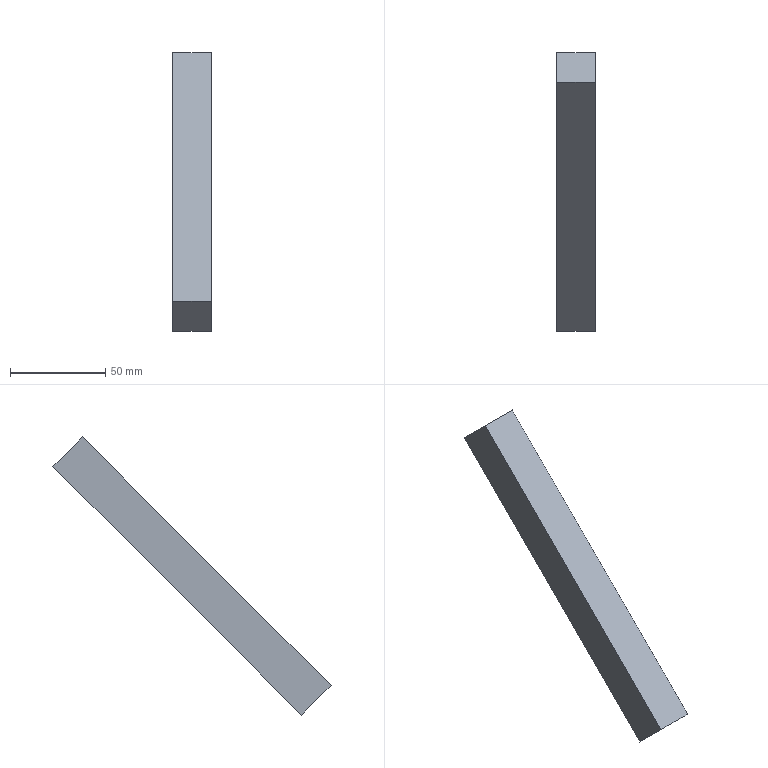Part | NX | features solid 2 | 1 solid | 6 faces | box 20 x 145.664 x 145.664 mm | volume 80960 mm3 | plane 6
STEP:
#1=CARTESIAN_POINT('',(-110.,-290.882,-104.607));
#2=VERTEX_POINT('',#1);
#3=CARTESIAN_POINT('',(-110.,-160.775,25.5));
#4=VERTEX_POINT('',#3);
#5=CARTESIAN_POINT('',(-110.,-282.751,-96.475));
#6=DIRECTION('',(0.,0.7071,0.7071));
#7=VECTOR('',#6,1000.);
#8=LINE('',#5,#7);
#9=EDGE_CURVE('',#2,#4,#8,.T.);
#10=ORIENTED_EDGE('',*,*,#9,.F.);
#11=CARTESIAN_POINT('',(-130.,-290.882,-104.607));
#12=VERTEX_POINT('',#11);
#13=CARTESIAN_POINT('',(-130.,-290.882,-104.607));
#14=DIRECTION('',(1.,0.,0.));
#15=VECTOR('',#14,1000.);
#16=LINE('',#13,#15);
#17=EDGE_CURVE('',#12,#2,#16,.T.);
#18=ORIENTED_EDGE('',*,*,#17,.F.);
#19=CARTESIAN_POINT('',(-130.,-160.775,25.5));
#20=VERTEX_POINT('',#19);
#21=CARTESIAN_POINT('',(-130.,-282.751,-96.475));
#22=DIRECTION('',(0.,0.7071,0.7071));
#23=VECTOR('',#22,1000.);
#24=LINE('',#21,#23);
#25=EDGE_CURVE('',#12,#20,#24,.T.);
#26=ORIENTED_EDGE('',*,*,#25,.T.);
#27=CARTESIAN_POINT('',(-130.,-160.775,25.5));
#28=DIRECTION('',(1.,0.,0.));
#29=VECTOR('',#28,1000.);
#30=LINE('',#27,#29);
#31=EDGE_CURVE('',#20,#4,#30,.T.);
#32=ORIENTED_EDGE('',*,*,#31,.T.);
#33=EDGE_LOOP('',(#10,#18,#26,#32));
#34=FACE_BOUND('',#33,.T.);
#35=CARTESIAN_POINT('',(-130.,-282.751,-96.475));
#36=DIRECTION('',(0.,0.7071,-0.7071));
#37=DIRECTION('',(0.,0.7071,0.7071));
#38=AXIS2_PLACEMENT_3D('',#35,#36,#37);
#39=PLANE('',#38);
#40=ADVANCED_FACE('',(#34),#39,.T.);
#41=CARTESIAN_POINT('',(-110.,-306.439,-89.051));
#42=VERTEX_POINT('',#41);
#43=CARTESIAN_POINT('',(-110.,-290.882,-104.607));
#44=DIRECTION('',(0.,-0.7071,0.7071));
#45=VECTOR('',#44,1000.);
#46=LINE('',#43,#45);
#47=EDGE_CURVE('',#2,#42,#46,.T.);
#48=ORIENTED_EDGE('',*,*,#47,.T.);
#49=CARTESIAN_POINT('',(-130.,-306.439,-89.051));
#50=VERTEX_POINT('',#49);
#51=CARTESIAN_POINT('',(-130.,-306.439,-89.051));
#52=DIRECTION('',(1.,0.,0.));
#53=VECTOR('',#52,1000.);
#54=LINE('',#51,#53);
#55=EDGE_CURVE('',#50,#42,#54,.T.);
#56=ORIENTED_EDGE('',*,*,#55,.F.);
#57=CARTESIAN_POINT('',(-130.,-290.882,-104.607));
#58=DIRECTION('',(0.,-0.7071,0.7071));
#59=VECTOR('',#58,1000.);
#60=LINE('',#57,#59);
#61=EDGE_CURVE('',#12,#50,#60,.T.);
#62=ORIENTED_EDGE('',*,*,#61,.F.);
#63=ORIENTED_EDGE('',*,*,#17,.T.);
#64=EDGE_LOOP('',(#48,#56,#62,#63));
#65=FACE_BOUND('',#64,.T.);
#66=CARTESIAN_POINT('',(-130.,-306.439,-89.051));
#67=DIRECTION('',(0.,0.7071,0.7071));
#68=DIRECTION('',(0.,-0.7071,0.7071));
#69=AXIS2_PLACEMENT_3D('',#66,#67,#68);
#70=PLANE('',#69);
#71=ADVANCED_FACE('',(#65),#70,.F.);
#72=CARTESIAN_POINT('',(-110.,-176.331,41.057));
#73=VERTEX_POINT('',#72);
#74=CARTESIAN_POINT('',(-110.,-298.307,-80.919));
#75=DIRECTION('',(0.,0.7071,0.7071));
#76=VECTOR('',#75,1000.);
#77=LINE('',#74,#76);
#78=EDGE_CURVE('',#42,#73,#77,.T.);
#79=ORIENTED_EDGE('',*,*,#78,.T.);
#80=CARTESIAN_POINT('',(-130.,-176.331,41.057));
#81=VERTEX_POINT('',#80);
#82=CARTESIAN_POINT('',(-130.,-176.331,41.057));
#83=DIRECTION('',(1.,0.,0.));
#84=VECTOR('',#83,1000.);
#85=LINE('',#82,#84);
#86=EDGE_CURVE('',#81,#73,#85,.T.);
#87=ORIENTED_EDGE('',*,*,#86,.F.);
#88=CARTESIAN_POINT('',(-130.,-298.307,-80.919));
#89=DIRECTION('',(0.,0.7071,0.7071));
#90=VECTOR('',#89,1000.);
#91=LINE('',#88,#90);
#92=EDGE_CURVE('',#50,#81,#91,.T.);
#93=ORIENTED_EDGE('',*,*,#92,.F.);
#94=ORIENTED_EDGE('',*,*,#55,.T.);
#95=EDGE_LOOP('',(#79,#87,#93,#94));
#96=FACE_BOUND('',#95,.T.);
#97=CARTESIAN_POINT('',(-130.,-298.307,-80.919));
#98=DIRECTION('',(0.,0.7071,-0.7071));
#99=DIRECTION('',(0.,0.7071,0.7071));
#100=AXIS2_PLACEMENT_3D('',#97,#98,#99);
#101=PLANE('',#100);
#102=ADVANCED_FACE('',(#96),#101,.F.);
#103=CARTESIAN_POINT('',(-110.,-160.775,25.5));
#104=DIRECTION('',(0.,-0.7071,0.7071));
#105=VECTOR('',#104,1000.);
#106=LINE('',#103,#105);
#107=EDGE_CURVE('',#4,#73,#106,.T.);
#108=ORIENTED_EDGE('',*,*,#107,.F.);
#109=ORIENTED_EDGE('',*,*,#31,.F.);
#110=CARTESIAN_POINT('',(-130.,-160.775,25.5));
#111=DIRECTION('',(0.,-0.7071,0.7071));
#112=VECTOR('',#111,1000.);
#113=LINE('',#110,#112);
#114=EDGE_CURVE('',#20,#81,#113,.T.);
#115=ORIENTED_EDGE('',*,*,#114,.T.);
#116=ORIENTED_EDGE('',*,*,#86,.T.);
#117=EDGE_LOOP('',(#108,#109,#115,#116));
#118=FACE_BOUND('',#117,.T.);
#119=CARTESIAN_POINT('',(-130.,-176.331,41.057));
#120=DIRECTION('',(0.,0.7071,0.7071));
#121=DIRECTION('',(0.,-0.7071,0.7071));
#122=AXIS2_PLACEMENT_3D('',#119,#120,#121);
#123=PLANE('',#122);
#124=ADVANCED_FACE('',(#118),#123,.T.);
#125=ORIENTED_EDGE('',*,*,#25,.F.);
#126=ORIENTED_EDGE('',*,*,#61,.T.);
#127=ORIENTED_EDGE('',*,*,#92,.T.);
#128=ORIENTED_EDGE('',*,*,#114,.F.);
#129=EDGE_LOOP('',(#125,#126,#127,#128));
#130=FACE_BOUND('',#129,.T.);
#131=CARTESIAN_POINT('',(-130.,-282.751,-96.475));
#132=DIRECTION('',(1.,0.,0.));
#133=DIRECTION('',(0.,0.9659,0.2588));
#134=AXIS2_PLACEMENT_3D('',#131,#132,#133);
#135=PLANE('',#134);
#136=ADVANCED_FACE('',(#130),#135,.F.);
#137=ORIENTED_EDGE('',*,*,#9,.T.);
#138=ORIENTED_EDGE('',*,*,#107,.T.);
#139=ORIENTED_EDGE('',*,*,#78,.F.);
#140=ORIENTED_EDGE('',*,*,#47,.F.);
#141=EDGE_LOOP('',(#137,#138,#139,#140));
#142=FACE_BOUND('',#141,.T.);
#143=CARTESIAN_POINT('',(-110.,-282.751,-96.475));
#144=DIRECTION('',(1.,0.,0.));
#145=DIRECTION('',(0.,0.9659,0.2588));
#146=AXIS2_PLACEMENT_3D('',#143,#144,#145);
#147=PLANE('',#146);
#148=ADVANCED_FACE('',(#142),#147,.T.);
#149=CLOSED_SHELL('',(#40,#71,#102,#124,#136,#148));
#150=MANIFOLD_SOLID_BREP('',#149);
#151=(LENGTH_UNIT()NAMED_UNIT(*)SI_UNIT(.MILLI.,.METRE.));
#152=UNCERTAINTY_MEASURE_WITH_UNIT(LENGTH_MEASURE(0.00001),#151,'','');
#153=(NAMED_UNIT(*)PLANE_ANGLE_UNIT()SI_UNIT($,.RADIAN.));
#154=(NAMED_UNIT(*)SI_UNIT($,.STERADIAN.)SOLID_ANGLE_UNIT());
#155=(GEOMETRIC_REPRESENTATION_CONTEXT(3)GLOBAL_UNCERTAINTY_ASSIGNED_CONTEXT((#152))GLOBAL_UNIT_ASSIGNED_CONTEXT((#151,#153,#154))REPRESENTATION_CONTEXT('',''));
#156=ADVANCED_BREP_SHAPE_REPRESENTATION('',(#150),#155);